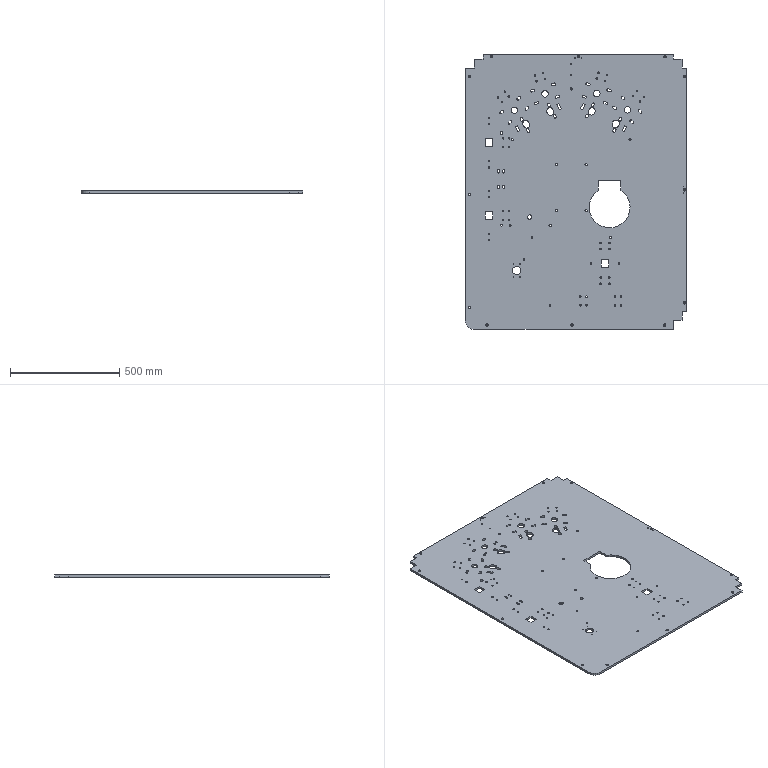Part | 1 solid | 436 faces | box 1016 x 1260 x 10 mm | volume 12181189 mm3 | cylinder 307 | plane 129 | commonest cylinder face diameters 6.8 x118 10 x52 8 x24 11 x24 12 x24 30 x20